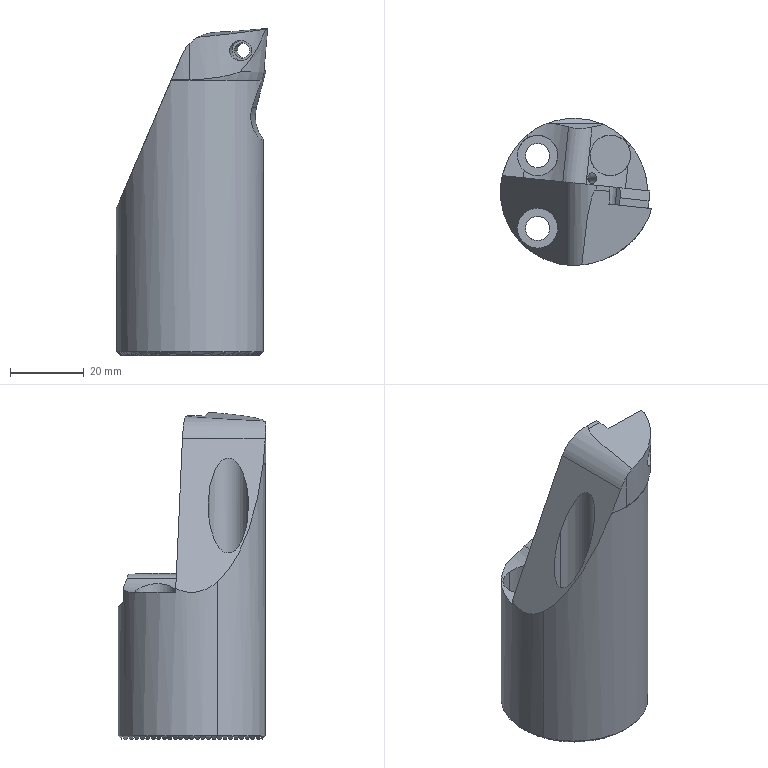NC program | Mastercam | posted with a generic post
Lines 3214 to 3959 of 11394:
(12 FEMR |TOOL - 1|DIA. OFF. - 1|LEN. - 1|TOOL DIA. - 12.)
N6488 T1 M6
N6490 G0 G55 G90 X52.429 Y2.915 C6. B-90. S3500 M3
N6492 G43 H1 Z102.44
N6494 Z4.44
N6496 G1 Z2.69 F2000.
N6498 X51.709 Y1.202 Z2.534 F2800.
N6500 G3 X51.498 Y.155 Z2.444 I2.488 J-1.047
N6502 G1 Y.102 Z2.44
N6504 G2 X51.5 Y-.095 I-12.825 J-.197
N6506 X51.357 Y-1.997 I-12.827
N6508 G3 X51.22 Y-5.555 I46.032 J-3.558
N6510 G1 Y-5.6
N6512 G3 X51.199 Y-11.817 I919.985 J-6.217
N6514 X51.2 Y-13.276 I920.006
N6516 G1 Y-13.683
N6518 X51.199 Y-18.228
N6520 G2 X50.215 Y-21.444 I-6.266 J.16
N6522 X47.628 Y-23.929 I-6.46 J4.134
N6524 X46.5 Y-24.503 I-4.781 J8.001
N6526 G1 Y-24.91
N6528 Y-25.317
N6530 G3 X48.731 Y-27.976 Z2.69 I2.7
N6532 X49.2 Y-28.017 I.469 J2.659
N6534 X51.844 Y-25.863 J2.7
N6536 G1 X56.791 Y-1.897 F9500.
N6538 G3 X56.847 Y-1.351 I-2.644 J.546
N6540 X54.147 Y1.349 I-2.7
N6542 X53.91 Y1.339 J-2.7
N6544 X51.457 Y-1.117 Z2.44 I.237 J-2.69 F2800.
N6546 G2 X51.192 Y-2.799 I-13.445 J1.253
N6548 G3 X50.977 Y-5.337 I20.312 J-3.005
N6550 X50.9 Y-11.409 I240.482 J-6.072
N6552 X50.902 Y-12.47 I240.559
N6554 G1 Y-12.876
N6556 X50.898 Y-16.434
N6558 G2 X49.12 Y-21.352 I-8.034 J.124
N6560 X47.471 Y-23.101 I-10.884 J8.606
N6562 X46.91 Y-23.542 I-5.216 J6.064
N6564 G3 X46.5 Y-24.082 I.712 J-.966
N6566 G1 X47.429 Y-24.318 Z2.503
N6568 G3 X48.094 Y-24.401 Z2.548 I.665 J2.617
N6570 X50.016 Y-23.596 Z2.69 J2.7
N6572 X50.662 Y-22.535 I-1.922 J1.895 F9500.
N6574 G1 X57.253 Y-2.23
N6576 G3 X57.385 Y-1.396 I-2.568 J.834
N6578 X54.685 Y1.304 I-2.7
N6580 X53.472 Y1.016 J-2.7
N6582 X52.427 Y.085 Z2.596 I1.213 J-2.412 F2800.
N6584 G1 X51.755 Y-.941 Z2.514
N6586 G3 X51.348 Y-1.984 Z2.44 I2.258 J-1.48
N6588 G2 X50.984 Y-3.578 I-14.281 J2.421
N6590 G3 X50.718 Y-6.011 I16.926 J-3.085
N6592 X50.606 Y-11.667 I142.458 J-5.656
N6594 X50.607 Y-12.256 I142.57
N6596 X50.603 Y-13.875 I988.13 J-3.02
N6598 G2 X50.606 Y-14.243 I-20.498 J-.368
N6600 X50.524 Y-16.082 I-20.501
N6602 X48.632 Y-20.865 I-10.086 J1.224
N6604 X47.071 Y-22.755 I-15.49 J11.204
N6606 G3 X46.616 Y-23.279 I1.242 J-1.538
N6608 X46.5 Y-23.627 I1.067 J-.549
N6610 G1 X47.429 Y-23.722 Z2.502
N6612 G3 X47.705 Y-23.736 Z2.52 I.276 J2.685
N6614 X49.898 Y-22.611 Z2.69 J2.699
N6616 X50.238 Y-21.97 I-2.193 J1.574 F9500.
N6618 G1 X57.092 Y-3.365
N6620 G3 X57.259 Y-2.431 I-2.534 J.934
N6622 X54.558 Y.27 I-2.701
N6624 X53.519 Y.061 J-2.701
N6626 X52.411 Y-.795 Z2.596 I1.039 J-2.492 F2800.
N6628 G1 X51.668 Y-1.77 Z2.514
N6630 G3 X51.188 Y-2.782 Z2.44 I2.147 J-1.637
N6632 G2 X50.81 Y-4.078 I-14.826 J3.626
N6634 G3 X50.481 Y-6.321 I12.813 J-3.026
N6636 X50.319 Y-11.538 I83.903 J-5.217
N6638 G1 Y-11.649
N6640 G3 X50.311 Y-12.86 I419.156 J-3.284
N6642 G2 X50.314 Y-13.177 I-17.115 J-.317
N6644 X50.129 Y-15.683 I-17.118
N6646 X48.043 Y-20.74 I-12.087 J2.027
N6648 X46.907 Y-22.292 I-23.75 J16.204
N6650 G3 X46.5 Y-22.983 I.919 J-1.006
N6652 X46.89 Y-23.011 Z2.466 I.39 J2.671
N6654 X49.383 Y-21.348 Z2.676 J2.699
N6656 G1 X49.46 Y-21.163 Z2.69
N6658 X56.133 Y-5.11 F9500.
N6660 G3 X56.34 Y-4.074 I-2.494 J1.036
N6662 X53.929 Y-1.389 I-2.701
N6664 X53.639 Y-1.373 Z2.671 I-.29 J-2.685 F2800.
N6666 X51.046 Y-3.322 Z2.44 J-2.701
N6668 G2 X50.627 Y-4.54 I-14.301 J4.235
N6670 G3 X50.248 Y-6.638 I10.5 J-2.983
N6672 X50.042 Y-11.072 I55.575 J-4.805
N6674 G1 X50.035 Y-11.471
N6676 Y-11.548
N6678 G2 X49.879 Y-14.469 I-27.299
N6680 X48.035 Y-19.837 I-13.828 J1.75
N6682 X46.726 Y-21.902 I-38.46 J22.916
N6684 G3 X46.5 Y-22.603 I.974 J-.701
N6686 X48.731 Y-25.262 Z2.69 I2.7
N6688 X49.2 Y-25.303 I.469 J2.659 F9500.
N6690 X51.827 Y-23.226 J2.7
N6692 G1 X56.076 Y-5.301
N6694 G3 X56.149 Y-4.679 I-2.627 J.622
N6696 X53.858 Y-2.01 I-2.7
N6698 X53.449 Y-1.979 Z2.663 I-.409 J-2.669 F2800.
N6700 X50.892 Y-3.812 Z2.44 J-2.7
N6702 G2 X50.448 Y-4.944 I-13.452 J4.631
N6704 G3 X50.023 Y-6.906 I8.754 J-2.922
N6706 X49.768 Y-10.878 I41.358 J-4.645
N6708 G2 X49.571 Y-13.811 I-30.227 J.564
N6710 X47.805 Y-19.31 I-15.936 J2.082
N6712 X46.648 Y-21.428 I-79.522 J42.076
N6714 G3 X46.5 Y-22.006 I1.052 J-.578
N6716 G1 Y-22.413
N6718 G3 X48.731 Y-25.071 Z2.69 I2.7
N6720 X49.2 Y-25.112 I.469 J2.658 F9500.
N6722 X51.828 Y-23.032 J2.699
N6724 G1 X55.885 Y-5.831
N6726 G3 X55.957 Y-5.211 I-2.628 J.62
N6728 X53.772 Y-2.56 I-2.7
N6730 X53.257 Y-2.51 Z2.656 I-.515 J-2.651 F2800.
N6732 X50.736 Y-4.243 Z2.44 J-2.701
N6734 G2 X50.26 Y-5.33 I-13.117 J5.108
N6736 G3 X49.798 Y-7.186 I7.651 J-2.887
N6738 X49.519 Y-10.342 I32.048 J-4.43
N6740 G2 X49.201 Y-13.711 I-33.187 J1.43
N6742 X47.544 Y-18.895 I-18.539 J3.068
N6744 X46.991 Y-20.043 I-62.668 J29.505
N6746 G3 X46.617 Y-20.853 I35.465 J-16.864
N6748 X46.5 Y-21.369 I1.083 J-.516
N6750 G1 Y-21.776
N6752 G3 X48.731 Y-24.435 Z2.69 I2.7
N6754 X49.2 Y-24.476 I.469 J2.659 F9500.
N6756 X51.826 Y-22.406 J2.7
N6758 G1 X55.678 Y-6.344
N6760 G3 X55.753 Y-5.714 I-2.625 J.63
N6762 X53.669 Y-3.085 I-2.7
N6764 X53.053 Y-3.014 Z2.649 I-.616 J-2.629 F2800.
N6766 X50.571 Y-4.651 Z2.44 J-2.7
N6768 G2 X50.073 Y-5.68 I-12.617 J5.47
N6770 G3 X49.578 Y-7.441 I6.759 J-2.849
N6772 X49.261 Y-10.214 I30.825 J-4.933
N6774 G2 X48.749 Y-14.057 I-30.915 J2.158
N6776 X47.32 Y-18.45 I-22.243 J4.808
N6778 G3 X46.572 Y-20.279 I24.909 J-11.252
N6780 X46.5 Y-20.689 I1.128 J-.41
N6782 G1 Y-21.096
N6784 G3 X48.731 Y-23.755 Z2.69 I2.7
N6786 X49.2 Y-23.796 I.469 J2.659 F9500.
N6788 X51.823 Y-21.737 J2.7
N6790 G1 X55.47 Y-6.813
N6792 G3 X55.547 Y-6.172 I-2.623 J.641
N6794 X53.555 Y-3.567 I-2.7
N6796 X52.847 Y-3.473 Z2.642 I-.708 J-2.605 F2800.
N6798 X50.404 Y-5.022 Z2.44 J-2.699
N6800 G2 X49.872 Y-6.031 I-13.084 J6.253
N6802 G3 X49.349 Y-7.741 I6.327 J-2.873
N6804 X48.951 Y-10.584 I38.683 J-6.863
N6806 G2 X48.011 Y-15.399 I-28.238 J3.012
N6808 X46.814 Y-18.791 I-45.682 J14.209
N6810 G3 X46.553 Y-19.565 I11.229 J-4.226
N6812 X46.499 Y-19.941 I1.272 J-.376
N6814 X46.5 Y-20.012 I1.326
N6816 G1 Y-20.419
N6818 G3 X48.731 Y-23.078 Z2.69 I2.7
N6820 X49.2 Y-23.119 I.469 J2.659 F9500.
N6822 X51.82 Y-21.07 J2.7
N6824 G1 X55.245 Y-7.274
N6826 G3 X55.325 Y-6.623 I-2.62 J.651
N6828 X53.425 Y-4.045 I-2.7
N6830 X52.625 Y-3.924 Z2.636 I-.8 J-2.578 F2800.
N6832 X50.224 Y-5.387 Z2.44 J-2.699
N6834 G2 X49.657 Y-6.382 I-14.741 J7.747
N6836 G3 X49.098 Y-8.108 I6.407 J-3.028
N6838 X48.6 Y-11.048 I58.68 J-11.445
N6840 G2 X46.971 Y-17.389 I-32.951 J5.087
N6842 G3 X46.542 Y-18.722 I21.473 J-7.64
N6844 X46.5 Y-19.039 I1.158 J-.317
N6846 G1 Y-19.445
N6848 Y-20.419
N6850 G3 X48.731 Y-23.078 Z2.69 I2.7
N6852 X49.2 Y-23.119 I.469 J2.659 F9500.
N6854 X51.826 Y-21.046 J2.7
N6856 G1 X55.013 Y-7.693
N6858 G3 X55.087 Y-7.066 I-2.626 J.627
N6860 X53.278 Y-4.517 I-2.7
N6862 X52.387 Y-4.366 Z2.63 I-.891 J-2.549 F2800.
N6864 X50.032 Y-5.746 Z2.44 J-2.7
N6866 G2 X49.427 Y-6.731 I-9.962 J5.428
N6868 G3 X48.894 Y-8.231 I6.052 J-2.996
N6870 X48.299 Y-11.118 I51.822 J-12.187
N6872 G2 X46.831 Y-16.771 I-43.565 J8.299
N6874 G3 X46.538 Y-17.769 I17.962 J-5.809
N6876 X46.5 Y-18.07 I1.162 J-.301
N6878 G1 Y-18.477
N6880 Y-19.698
N6882 G3 X48.731 Y-22.357 Z2.69 I2.7
N6884 X49.2 Y-22.398 I.469 J2.659 F9500.
N6886 X51.825 Y-20.329 J2.7
N6888 G1 X54.758 Y-8.131
N6890 G3 X54.833 Y-7.5 I-2.625 J.631
N6892 X53.114 Y-4.984 I-2.7
N6894 X52.133 Y-4.8 Z2.623 I-.981 J-2.516 F2800.
N6896 X49.826 Y-6.097 Z2.44 J-2.7
N6898 G2 X49.26 Y-6.942 I-9.826 J5.974
N6900 G3 X48.684 Y-8.373 I5.52 J-3.053
N6902 X47.999 Y-11.192 I43.696 J-12.109
N6904 G2 X46.685 Y-16.178 I-68.436 J15.375
N6906 G3 X46.538 Y-16.724 I15.502 J-4.456
N6908 X46.5 Y-17.024 I1.162 J-.3
N6910 G1 Y-17.431
N6912 Y-18.652
N6914 G3 X48.731 Y-21.31 Z2.69 I2.7
N6916 X49.2 Y-21.351 I.469 J2.658 F9500.
N6918 X51.82 Y-19.302 J2.699
N6920 G1 X54.485 Y-8.575
N6922 G3 X54.565 Y-7.924 I-2.62 J.651
N6924 X52.934 Y-5.445 I-2.7
N6926 X51.865 Y-5.224 Z2.617 I-1.069 J-2.479 F2800.
N6928 X49.609 Y-6.441 Z2.44 J-2.7
N6930 G2 X49.03 Y-7.244 I-9.609 J6.318
N6932 G3 X48.403 Y-8.716 I5.97 J-3.41
N6934 X47.531 Y-11.933 I52.222 J-15.888
N6936 G2 X46.535 Y-15.637 I-161.889 J41.54
N6938 G3 X46.5 Y-15.925 I1.165 J-.288
N6940 G1 Y-16.332
N6942 Y-17.553
N6944 G3 X48.731 Y-20.212 Z2.69 I2.7
N6946 X49.2 Y-20.253 I.469 J2.659 F9500.
N6948 X51.813 Y-18.232 J2.7
N6950 G1 X54.214 Y-8.991
N6952 G3 X54.301 Y-8.312 I-2.613 J.679
N6954 X52.751 Y-5.869 I-2.7
N6956 X51.601 Y-5.612 Z2.611 I-1.15 J-2.443 F2800.
N6958 X49.395 Y-6.755 Z2.44 J-2.7
N6960 G2 X48.815 Y-7.524 I-9.309 J6.421
N6962 G3 X48.151 Y-8.94 I5.556 J-3.467
N6964 X47.208 Y-12.058 I41.019 J-14.099
N6966 G1 X47.1 Y-12.449
N6968 G3 X46.535 Y-14.527 I79.743 J-22.772
N6970 X46.5 Y-14.816 I1.165 J-.289
N6972 G1 Y-15.223
N6974 Y-16.443
N6976 G3 X48.731 Y-19.102 Z2.69 I2.7
N6978 X49.2 Y-19.143 I.469 J2.659 F9500.
N6980 X51.798 Y-17.178 J2.7
N6982 G1 X54.034 Y-9.276
N6984 G3 X54.136 Y-8.541 I-2.598 J.735
N6986 X52.634 Y-6.122 I-2.7
N6988 X51.436 Y-5.842 Z2.608 I-1.198 J-2.419 F2800.
N6990 X49.261 Y-6.94 Z2.44 J-2.699
N6992 G2 X48.886 Y-7.422 I-9.261 J6.817
N6994 G3 X48.015 Y-8.867 I3.853 J-3.308
N6996 X47.023 Y-11.746 I24.798 J-10.157
N6998 X46.545 Y-13.426 I45.824 J-13.932
N7000 X46.493 Y-13.911 I2.231 J-.485
N7002 X46.5 Y-14.087 I2.283
N7004 G1 Y-14.494
N7006 Y-15.308
N7008 G3 X48.731 Y-17.967 Z2.69 I2.7
N7010 X49.2 Y-18.008 I.469 J2.659 F9500.
N7012 X51.787 Y-16.082 J2.7
N7014 G1 X53.676 Y-9.766
N7016 G3 X53.789 Y-8.992 I-2.587 J.774
N7018 X52.384 Y-6.623 I-2.7
N7020 X51.089 Y-6.292 Z2.6 I-1.295 J-2.369 F2800.
N7022 X48.981 Y-7.306 Z2.44 J-2.7
N7024 G2 X48.886 Y-7.422 I-8.981 J7.183
N7026 G3 X47.284 Y-10.248 I6.632 J-5.628
N7028 X46.749 Y-11.814 I22.033 J-8.401
N7030 X46.5 Y-14.087 I10.251 J-2.273
N7032 X48.731 Y-16.746 Z2.69 I2.7
N7034 X49.2 Y-16.787 I.469 J2.659 F9500.
N7036 X51.783 Y-14.874 J2.7
N7038 G1 X53.108 Y-10.525
N7040 G3 X53.225 Y-9.738 I-2.583 J.787
N7042 X51.618 Y-7.269 I-2.7
N7044 X50.525 Y-7.038 Z2.615 I-1.093 J-2.469 F2800.
N7046 X48.284 Y-8.232 Z2.44 J-2.7
N7048 X46.678 Y-12.161 I8.716 J-5.855
N7050 X46.632 Y-12.656 Z2.473 I2.654 J-.495
N7052 X46.706 Y-13.28 Z2.514 I2.7
N7054 G1 X47.316 Y-15.851 Z2.69
N7056 X47.429 Y-16.325 F9500.
N7058 G3 X50.056 Y-18.4 I2.627 J.625
N7060 X52.756 Y-15.7 J2.7
N7062 G1 Y-15.691
N7064 X52.597 Y28.103
N7066 G3 X49.897 Y30.793 I-2.7 J-.01
N7068 X47.94 Y29.954 J-2.7
N7070 X47.429 Y29.188 Z2.628 I1.957 J-1.861 F2800.
N7072 G1 X46.732 Y27.619 Z2.514
N7074 G3 X46.5 Y26.523 Z2.44 I2.468 J-1.096
N7076 G1 Y25.913
N7078 Y25.798
N7080 G3 X47.406 Y25.127 I94.594 J126.953
N7082 G2 X50.012 Y21.693 I-5.149 J-6.612
N7084 X50.873 Y18.462 I-11.927 J-4.911
N7086 X51.15 Y14.618 I-33.704 J-4.353
N7088 X51.203 Y7.326 I-499.303 J-7.292
N7090 X51.2 Y5.532 I-499.356
N7092 G1 Y5.124
N7094 Y2.622
N7096 G3 X51.228 Y2.363 I1.2
N7098 G2 X51.5 Y-.059 I-11.228 J-2.486
N7100 G3 X53.746 Y-2.706 Z2.69 I2.7 J.014
N7102 X54.2 Y-2.744 I.454 J2.661
N7104 X56.899 Y-.045 J2.699
N7106 X56.852 Y.462 I-2.699
N7108 G1 X51.852 Y26.622 F9500.
N7110 G3 X49.2 Y28.815 I-2.652 J-.507
N7112 X48.731 Y28.774 J-2.7
N7114 X46.5 Y26.115 Z2.44 I.469 J-2.659 F2800.
N7116 G1 Y25.505
N7118 Y25.315
N7120 X47.627 Y24.147
N7122 G2 X49.95 Y19.933 I-8.334 J-7.342
N7124 X50.64 Y16.364 I-17.478 J-5.232
N7126 X50.87 Y11.435 I-56.298 J-5.095
N7128 X50.907 Y4.219 I-698.368 J-7.216
N7130 G1 Y3.68
N7132 G3 X50.963 Y3.351 I1.2 J.034
N7134 G2 X51.343 Y1.77 I-10.963 J-3.474
N7136 G3 X53.982 Y-.485 Z2.69 I2.663 J.444
N7138 G1 X54.006 F9500.
N7140 G3 X56.705 Y2.214 J2.699
N7142 X56.651 Y2.756 I-2.699
N7144 G1 X51.845 Y26.214
N7146 G3 X49.2 Y28.373 I-2.645 J-.541
N7148 X48.731 Y28.331 J-2.7
N7150 X46.5 Y25.673 Z2.44 I.469 J-2.658 F2800.
N7152 G1 Y25.062
N7154 Y24.856
N7156 X47.491 Y23.589
N7158 G2 X49.538 Y19.484 I-10.793 J-7.945
N7160 X50.33 Y15.29 I-20.604 J-6.065
N7162 X50.568 Y9.983 I-66.22 J-5.62
N7164 X50.607 Y4.795 I-432.577 J-5.898
N7166 G3 X50.606 Y4.746 I2.307 J-.049
N7168 X50.706 Y4.076 I2.308
N7170 G2 X51.091 Y2.918 I-10.706 J-4.199
N7172 G3 X53.695 Y.932 Z2.673 I2.604 J.714
N7174 X53.946 Y.943 Z2.69 J2.7
N7176 X56.396 Y3.632 I-.251 J2.689 F9500.
N7178 X56.338 Y4.182 I-2.701
N7180 G1 X51.843 Y25.788
N7182 G3 X49.2 Y27.938 I-2.643 J-.549
N7184 X48.731 Y27.898 J-2.699
N7186 X46.5 Y25.239 Z2.44 I.469 J-2.659 F2800.
N7188 G1 Y24.628
N7190 Y24.406
N7192 X47.405 Y23.017
N7194 G2 X49.537 Y17.659 I-14.214 J-8.759
N7196 X50.14 Y12.826 I-30.664 J-6.282
N7198 X50.289 Y6.512 I-134.002 J-6.314
N7200 G1 Y6.492
N7202 Y6.469
N7204 G3 X50.35 Y5.055 I16.422
N7206 X50.454 Y4.67 I1.194 J.116
N7208 G2 X50.903 Y3.536 I-10.454 J-4.793
N7210 G3 X53.462 Y1.696 Z2.663 I2.559 J.859
N7212 X53.864 Y1.725 Z2.69 J2.699
N7214 X56.162 Y4.395 I-.402 J2.67 F9500.
N7216 X56.105 Y4.947 I-2.7
N7218 G1 X51.843 Y25.358
N7220 G3 X49.2 Y27.506 I-2.643 J-.552
N7222 X48.731 Y27.465 J-2.7
N7224 X46.5 Y24.806 Z2.44 I.469 J-2.659 F2800.
N7226 G1 Y24.195
N7228 Y23.955
N7230 X47.461 Y22.188
N7232 G2 X49.416 Y16.074 I-18.276 J-9.214
N7234 X49.883 Y10.994 I-41.232 J-6.348
N7236 X49.986 Y6.875 I-170.329 J-6.326
N7238 G3 X50.078 Y5.577 I11.967 J.193
N7240 X50.202 Y5.184 I1.189 J.161
N7242 G2 X50.707 Y4.074 I-10.202 J-5.307
N7244 G3 X53.221 Y2.359 Z2.654 I2.514 J.985
N7246 X53.755 Y2.412 Z2.69 J2.7
N7248 X55.921 Y5.059 I-.534 J2.647 F9500.
N7250 X55.864 Y5.609 I-2.7
N7252 G1 X51.843 Y24.923
N7254 G3 X49.2 Y27.073 I-2.643 J-.55
N7256 X48.731 Y27.032 J-2.7
N7258 X46.5 Y24.373 Z2.44 I.469 J-2.659 F2800.
N7260 G1 Y23.762
N7262 Y23.493
N7264 X47.469 Y21.371
N7266 G2 X49.19 Y14.988 I-22.539 J-9.501
N7268 X49.602 Y9.587 I-52.121 J-6.697
N7270 X49.641 Y8.354 I-338.797 J-11.28
N7272 G3 X49.784 Y6.169 I20.974 J.273
N7274 X49.95 Y5.643 I1.348 J.137
N7276 G2 X50.505 Y4.556 I-9.95 J-5.766
N7278 G3 X52.972 Y2.954 Z2.646 I2.467 J1.099
N7280 X53.625 Y3.035 Z2.69 J2.701
N7282 X55.672 Y5.655 I-.653 J2.62 F9500.
N7284 X55.616 Y6.2 I-2.7
N7286 G1 X51.844 Y24.477
N7288 G3 X49.2 Y26.632 I-2.644 J-.545
N7290 X48.731 Y26.591 J-2.7
N7292 X46.5 Y23.932 Z2.44 I.469 J-2.659 F2800.
N7294 G1 Y23.321
N7296 Y23.015
N7298 X47.439 Y20.557
N7300 G2 X49.01 Y13.429 I-28.117 J-9.934
N7302 X49.319 Y8.675 I-75.002 J-7.272
N7304 G3 X49.509 Y6.581 I17.357 J.512
N7306 X49.697 Y6.06 I1.327 J.184
N7308 G2 X50.11 Y5.359 I-9.697 J-6.183
N7310 G3 X52.483 Y3.946 Z2.632 I2.373 J1.287
N7312 X53.338 Y4.085 Z2.69 J2.7
N7314 X55.183 Y6.646 I-.855 J2.561 F9500.
N7316 X55.133 Y7.163 I-2.7
N7318 G1 X51.85 Y23.994
N7320 G3 X49.2 Y26.177 I-2.65 J-.517
N7322 X48.731 Y26.136 J-2.7
N7324 X46.5 Y23.477 Z2.44 I.469 J-2.659 F2800.
N7326 G1 Y22.866
N7328 Y22.508
N7330 X47.381 Y19.732
N7332 G2 X48.764 Y12.327 I-34.511 J-10.274
N7334 X49.024 Y8.609 I-130.35 J-10.996
N7336 G3 X49.26 Y6.846 I11.248 J.607
N7338 X49.441 Y6.444 I1.166 J.283
N7340 G2 X49.882 Y5.76 I-9.441 J-6.567
N7342 G3 X52.202 Y4.441 Z2.625 I2.32 J1.381
N7344 X53.159 Y4.616 Z2.69 J2.7
N7346 X54.902 Y7.141 I-.957 J2.525 F9500.
N7348 X54.855 Y7.643 I-2.7
N7350 G1 X51.853 Y23.501
N7352 G3 X49.2 Y25.699 I-2.653 J-.502
N7354 X48.731 Y25.658 J-2.7
N7356 X46.5 Y22.999 Z2.44 I.469 J-2.659 F2800.
N7358 G1 Y22.388
N7360 Y21.982
N7362 X47.505 Y18.044
N7364 G2 X48.514 Y11.273 I-43.491 J-9.938
N7366 G3 X48.781 Y8.274 I73.964 J5.078
N7368 X48.985 Y7.203 I7.419 J.856
N7370 X49.183 Y6.8 I1.156 J.319
N7372 G2 X49.65 Y6.133 I-9.183 J-6.923
N7374 G3 X51.915 Y4.902 Z2.618 I2.265 J1.469
N7376 X52.968 Y5.115 Z2.69 J2.7
N7378 X54.616 Y7.602 I-1.053 J2.487 F9500.
N7380 X54.572 Y8.086 I-2.701
N7382 G1 X51.856 Y22.981
N7384 G3 X49.2 Y25.197 I-2.656 J-.484
N7386 X48.731 Y25.156 J-2.7
N7388 X46.5 Y22.497 Z2.44 I.469 J-2.659 F2800.
N7390 G1 Y21.886
N7392 G3 X46.493 Y21.683 I3.128 J-.203
N7394 X46.592 Y20.904 I3.135
N7396 X47.243 Y17.821 I129.499 J25.759
N7398 G2 X48.229 Y10.819 I-56.073 J-11.469
N7400 G3 X48.559 Y8.123 I28.374 J2.104
N7402 X48.705 Y7.545 I5.317 J1.031
N7404 X48.924 Y7.131 I1.15 J.343
N7406 G2 X49.414 Y6.482 I-8.924 J-7.254
N7408 G3 X51.624 Y5.333 Z2.612 I2.21 J1.551
N7410 X52.768 Y5.587 Z2.69 J2.7
N7412 X54.324 Y8.033 I-1.144 J2.446 F9500.
N7414 X54.285 Y8.495 I-2.7
N7416 G1 X51.86 Y22.443
N7418 G3 X49.2 Y24.68 I-2.66 J-.463
N7420 X48.731 Y24.639 J-2.7
N7422 X46.5 Y21.98 Z2.44 I.469 J-2.659 F2800.
N7424 G1 Y21.37
N7426 Y21.285
N7428 G3 X46.665 Y19.533 I9.379
N7430 X47.213 Y16.354 I190.62 J31.235
N7432 G2 X47.918 Y10.831 I-84.144 J-13.541
N7434 G3 X48.298 Y8.293 I20.903 J1.839
N7436 X48.588 Y7.557 I2.045 J.381
N7438 X49.139 Y6.858 I32.356 J24.914
N7440 X51.285 Y5.797 Z2.604 I2.146 J1.639
N7442 X52.526 Y6.099 Z2.69 J2.7
N7444 X53.985 Y8.497 I-1.241 J2.398 F9500.
N7446 X53.95 Y8.927 I-2.7
N7448 G1 X51.865 Y21.841
N7450 G3 X49.2 Y24.11 I-2.665 J-.43
N7452 X48.731 Y24.07 J-2.699
N7454 X46.5 Y21.411 Z2.44 I.469 J-2.659 F2800.
N7456 G1 Y20.801
N7458 G3 X46.495 Y20.406 I14.528 J-.395
N7460 X46.667 Y18.174 I14.533
N7462 X47.06 Y15.383 I284.246 J38.655
N7464 G2 X47.66 Y10.514 I-184.401 J-25.163
N7466 G3 X48.056 Y8.423 I13.407 J1.459
N7468 X48.199 Y8.115 I1.149 J.346
N7470 X48.886 Y7.177 I8.801 J5.727
N7472 X50.973 Y6.19 Z2.598 I2.087 J1.714
N7474 X52.298 Y6.538 Z2.69 J2.701
N7476 X53.673 Y8.891 I-1.325 J2.353 F9500.
N7478 X53.642 Y9.294 I-2.7
N7480 G1 X51.87 Y21.014
N7482 G3 X49.2 Y23.31 I-2.67 J-.404
N7484 X48.731 Y23.269 J-2.7
N7486 X46.5 Y20.61 Z2.44 I.469 J-2.659 F2800.
N7488 G1 Y20.
N7490 G3 X46.498 Y19.584 I54.027 J-.416
N7492 X46.522 Y17.999 I54.029
N7494 X46.915 Y14.25 I79.496 J6.435
N7496 G1 X46.962 Y13.844
N7498 G3 X47.449 Y10.09 I80.041 J8.474
N7500 X47.646 Y9.141 I11.143 J1.824
N7502 X47.753 Y8.868 I1.163 J.296
N7504 X48.632 Y7.5 I9.247 J4.974
N7506 X50.783 Y6.432 Z2.605 I2.151 J1.631
N7508 G1 X51.102 Y6.45 Z2.626
N7510 X51.417 Y6.507 Z2.647
N7512 X51.723 Y6.6 Z2.669
N7514 X52.015 Y6.729 Z2.69
N7516 G3 X53.484 Y9.131 I-1.233 J2.403 F9500.
N7518 X53.45 Y9.551 I-2.701
N7520 G1 X51.867 Y19.595
N7522 G3 X49.2 Y21.875 I-2.667 J-.42
N7524 X48.731 Y21.834 J-2.7
N7526 X46.5 Y19.175 Z2.44 I.469 J-2.659 F2800.
N7528 G1 Y18.564
N7530 G3 X46.498 Y17.953 I80.546 J-.611
N7532 X46.523 Y15.941 I80.548
N7534 X47.173 Y10.209 I55.983 J3.444
N7536 X47.398 Y9.592 I2.118 J.426
N7538 X47.956 Y8.507 I9.602 J4.25
N7540 X50.282 Y7.179 Z2.626 I2.326 J1.372
N7542 X51.229 Y7.35 Z2.69 J2.7
N7544 X52.982 Y9.879 I-.947 J2.529 F9500.
N7546 X52.952 Y10.275 I-2.7
N7548 G1 X51.871 Y17.572
N7550 G3 X49.2 Y19.876 I-2.671 J-.396
N7552 X48.731 Y19.835 J-2.7
N7554 X46.5 Y17.176 Z2.44 I.469 J-2.659 F2800.
N7556 G1 Y16.566
N7558 G3 X46.497 Y15.753 I98.014 J-.813
N7560 X46.52 Y13.604 I98.017
N7562 X46.644 Y12.111 I22.902 J1.142
N7564 X47.486 Y9.399 I10.356 J1.731
N7566 X49.933 Y7.841 Z2.643 I2.447 J1.142
N7568 X50.633 Y7.934 Z2.69 J2.7
N7570 X52.632 Y10.541 I-.7 J2.607 F9500.
N7572 X52.594 Y10.996 I-2.699
N7574 G1 X51.861 Y15.287
N7576 G3 X49.2 Y17.532 I-2.661 J-.454
N7578 X48.731 Y17.492 J-2.699
N7580 X46.5 Y14.833 Z2.44 I.469 J-2.659 F2800.
N7582 G1 Y14.223
N7584 G3 X46.496 Y13.927 I11.092 J-.296
N7586 X46.783 Y11.422 I11.096
N7588 X47.992 Y9.746 Z2.634 I2.627 J.622
N7590 G1 X48.507 Y9.428 Z2.69
N7592 G0 Z102.44
N7594 X66.284 Y32.617
N7596 Z52.34
N7598 Z3.34
N7600 G1 Z-12.66 F2000.
N7602 G41 D1 X61.84 Y27.209 F1500.
N7604 G3 X61.795 Y27.082 I.155 J-.127
N7606 X61.868 Y26.927 I.2
N7608 G1 X63.413 Y25.657
N7610 G3 X65. Y25.089 I1.587 J1.932
N7612 X65.647 Y25.174 J2.5
N7614 G1 X75.181 Y27.729
N7616 X77.113 Y28.246
N7618 G3 X77.261 Y28.439 I-.052 J.193
N7620 X77.255 Y28.491 I-.2
N7622 G1 G40 X75.443 Y35.253
N7624 G0 Z37.34
N7626 X66.094 Y32.385
N7628 Z3.34
N7630 G1 Z-12.66 F2000.
N7632 G41 D1 X61.65 Y26.977 F1500.
N7634 G3 X61.604 Y26.85 I.154 J-.127
N7636 X61.677 Y26.695 I.2
N7638 G1 X63.222 Y25.425
N7640 G3 X65. Y24.788 I1.778 J2.164
N7642 X65.725 Y24.884 J2.801
N7644 G1 X75.259 Y27.439
N7646 X77.191 Y27.957
N7648 G3 X77.339 Y28.15 I-.052 J.193
N7650 X77.332 Y28.201 I-.2
N7652 G1 G40 X75.52 Y34.963
N7654 G0 Z37.34
N7656 X65.903 Y32.153
N7658 Z3.34
N7660 G1 Z-12.66 F2000.
N7662 G41 D1 X61.459 Y26.745 F1500.
N7664 G3 X61.414 Y26.618 I.155 J-.127
N7666 X61.487 Y26.463 I.2
N7668 G1 X63.032 Y25.194
N7670 G3 X65. Y24.489 I1.968 J2.395
N7672 X65.802 Y24.594 J3.1
N7674 G1 X75.337 Y27.149
N7676 X77.268 Y27.667
N7678 G3 X77.417 Y27.86 I-.051 J.193
N7680 X77.41 Y27.912 I-.2
N7682 G1 G40 X75.598 Y34.673
N7684 G0 Z37.34
N7686 X65.713 Y31.921
N7688 Z3.34
N7690 G1 Z-12.66 F2000.
N7692 G41 D1 X61.269 Y26.513 F1500.
N7694 G3 X61.223 Y26.386 I.154 J-.127
N7696 X61.296 Y26.232 I.2
N7698 G1 X62.841 Y24.962
N7700 G3 X65. Y24.189 I2.159 J2.627
N7702 X65.88 Y24.305 J3.4
N7704 G1 X75.414 Y26.859
N7706 X77.346 Y27.377
N7708 G3 X77.494 Y27.57 I-.052 J.193
N7710 X77.487 Y27.622 I-.2
N7712 G1 G40 X75.676 Y34.383
N7714 G0 Z37.34
N7716 X65.522 Y31.69
N7718 Z3.34
N7720 G1 Z-12.66 F2000.
N7722 G41 D1 X61.078 Y26.281 F1500.
N7724 G3 X61.033 Y26.154 I.155 J-.127
N7726 X61.106 Y26. I.2
N7728 G1 X62.651 Y24.73
N7730 G3 X65. Y23.889 I2.349 J2.859
N7732 X65.958 Y24.015 J3.7
N7734 G1 X75.492 Y26.57
N7736 X77.424 Y27.087
N7738 G3 X77.572 Y27.28 I-.052 J.193
N7740 X77.565 Y27.332 I-.2
N7742 G1 G40 X75.753 Y34.094
N7744 G0 Z37.34
N7746 X65.332 Y31.458
N7748 Z3.34
N7750 G1 Z-12.66 F2000.
N7752 G41 D1 X60.888 Y26.05 F1500.
N7754 G3 X60.842 Y25.923 I.154 J-.127
N7756 X60.915 Y25.768 I.2
N7758 G1 X62.46 Y24.498
N7760 G3 X65. Y23.588 I2.54 J3.091
N7762 X66.035 Y23.725 J4.001
N7764 G1 X75.569 Y26.28
N7766 X77.501 Y26.797
N7768 G3 X77.651 Y26.991 I-.051 J.194
N7770 X77.643 Y27.042 I-.201
N7772 G1 G40 X75.831 Y33.804
N7774 G0 Z52.34
N7776 Z52.84
N7778 X46.3 Y32.
N7780 Z3.84
N7782 G1 Z2.84 F2000.
N7784 G41 D1 Y20. F600.
N7786 Y13.842
N7788 G3 X48.732 Y7.05 I10.7
N7790 G2 X51.3 Y-.123 I-8.732 J-7.173
N7792 X48.732 Y-7.295 I-11.3
N7794 G3 X46.3 Y-14.087 I8.268 J-6.792
N7796 G1 Y-20.
N7798 G40 Y-32.
N7800 G0 Z52.84
N7802 X46.1 Y32.
N7804 Z3.84
N7806 G1 Z2.84 F2000.
N7808 G41 D1 Y20. F600.
N7810 Y13.842
N7812 G3 X48.577 Y6.923 I10.9
N7814 G2 X51.1 Y-.123 I-8.577 J-7.046
N7816 X48.577 Y-7.168 I-11.1
N7818 G3 X46.1 Y-14.087 I8.423 J-6.919
N7820 G1 Y-20.
N7822 G40 Y-32.
N7824 G0 Z52.84
N7826 Z70.5
N7828 X43.5 Y15.599
N7830 C0.
N7832 Z21.5
N7834 G1 Z20.025 F2000.
N7836 G41 D1 Y7.599 F1500.
N7838 Y-7.599
N7840 G40 Y-15.599
N7842 Z19.55 F2000.
N7844 G42 D1 Y-7.599 F1500.
N7846 Y7.599
N7848 G40 Y15.599
N7850 Z19.075 F2000.
N7852 G41 D1 Y7.599 F1500.
N7854 Y-7.599
N7856 G40 Y-15.599
N7858 Z18.6 F2000.
N7860 G42 D1 Y-7.599 F1500.
N7862 Y7.599
N7864 G40 Y15.599
N7866 G0 Z70.5
N7868 Z120.
N7870 X-43.576 Y-31.621
N7872 B-270.
N7874 Z22.
N7876 G1 Z-5.65 F2000.
N7878 X-42.879 Y-30.052 Z-5.801 F2800.
N7880 G3 X-42.647 Y-28.956 Z-5.9 I-2.468 J1.096
N7882 G1 Y-28.346
N7884 X-42.903 Y-28.278
N7886 G3 X-45.413 Y-28.097 I-2.72 J-20.131
N7888 X-52.432 Y-28.043 I-7.019 J-457.417
N7890 X-54.219 Y-28.046 J-457.471
N7892 G1 X-54.626
N7894 X-89.193 Y-28.039
N7896 G2 X-92.307 Y-27.242 I.126 J6.974
N7898 X-94.99 Y-24.745 I3.684 J6.65
N7900 X-96.367 Y-21.462 I8.666 J5.565
N7902 X-96.841 Y-17.959 I19.39 J4.406
N7904 X-96.958 Y-12.91 I108.682 J5.049
N7906 X-96.957 Y-12.379 I108.799
N7908 X-96.962 Y-9.923 I969.849 J3.173
N7910 G1 Y-9.516
N7912 X-96.964 Y30.474
N7914 G3 X-97.143 Y31.106 I-1.2
N7916 G1 X-97.893 Y30.275 Z-5.826
N7918 G3 X-99.413 Y28.111 Z-5.65 I8.089 J-7.297
N7920 X-100.698 Y22.978 I9.609 J-5.133
N7922 X-100.685 Y22.456 I10.894
N7924 G1 X-98.542 Y-22.245 F9500.
N7926 G3 X-91.537 Y-29.481 I7.617 J.365
N7928 G1 X-46.176 Y-33.133
N7930 G3 X-45.966 Y-33.141 I.21 J2.607
N7932 X-44.091 Y-32.349 J2.615
N7934 X-43.576 Y-31.587 Z-5.711 I-1.875 J1.823 F2800.
N7936 G1 X-42.879 Y-30.018 Z-5.825
N7938 G3 X-42.647 Y-28.922 Z-5.9 I-2.468 J1.096
N7940 G1 Y-28.312
N7942 Y-28.287
N7944 G3 X-43.369 Y-28.088 I-1.184 J-2.895
N7946 X-46.248 Y-27.827 I-3.283 J-20.205
N7948 X-52.373 Y-27.746 I-6.125 J-231.975
N7950 X-53.378 Y-27.749 J-232.056
N7952 G1 X-53.784 Y-27.748
N7954 X-87.726 Y-27.737
N7956 G2 X-93.695 Y-24.873 I.21 J8.091
N7958 X-95.726 Y-21.12 I7.989 J6.747
N7960 X-96.445 Y-17.256 I17.616 J5.278
N7962 X-96.639 Y-12.378 I63.382 J4.971
N7964 X-96.664 Y-5.381 I970.561 J6.997
N7966 X-96.663 Y-3.773 I970.586
N7968 G1 Y-3.365
N7970 X-96.672 Y29.434
N7972 G3 X-96.755 Y30.427 I-10.793 J-.403
N7974 X-96.986 Y31.024 I-1.194 J-.12
N7976 G1 X-97.673 Y30.275 Z-5.833